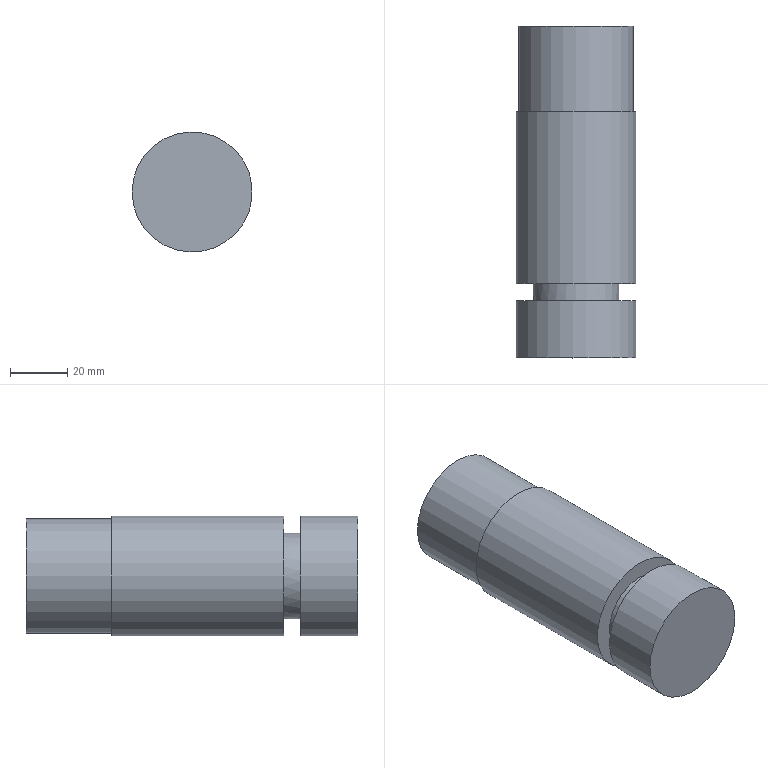Part | NX | features solid 2 | 1 solid | 9 faces | box 42 x 116 x 42 mm | volume 152776 mm3 | plane 5 | cylinder 4 | commonest cylinder face diameters 42 x2 30 x1 40 x1
STEP:
#1=CARTESIAN_POINT('',(-471.,-340.,180.));
#2=VERTEX_POINT('',#1);
#3=CARTESIAN_POINT('',(-450.,-340.,180.));
#4=DIRECTION('',(0.,1.,0.));
#5=DIRECTION('',(-1.,0.,0.));
#6=AXIS2_PLACEMENT_3D('',#3,#4,#5);
#7=CIRCLE('',#6,21.);
#8=EDGE_CURVE('',#2,#2,#7,.T.);
#9=ORIENTED_EDGE('',*,*,#8,.T.);
#10=EDGE_LOOP('',(#9));
#11=FACE_BOUND('',#10,.T.);
#12=CARTESIAN_POINT('',(-470.,-340.,180.));
#13=VERTEX_POINT('',#12);
#14=CARTESIAN_POINT('',(-450.,-340.,180.));
#15=DIRECTION('',(0.,1.,0.));
#16=DIRECTION('',(-1.,0.,0.));
#17=AXIS2_PLACEMENT_3D('',#14,#15,#16);
#18=CIRCLE('',#17,20.);
#19=EDGE_CURVE('',#13,#13,#18,.T.);
#20=ORIENTED_EDGE('',*,*,#19,.F.);
#21=EDGE_LOOP('',(#20));
#22=FACE_BOUND('',#21,.T.);
#23=CARTESIAN_POINT('',(-450.,-340.,180.));
#24=DIRECTION('',(0.,1.,0.));
#25=DIRECTION('',(0.,0.,1.));
#26=AXIS2_PLACEMENT_3D('',#23,#24,#25);
#27=PLANE('',#26);
#28=ADVANCED_FACE('',(#11,#22),#27,.T.);
#29=CARTESIAN_POINT('',(-471.,-400.,180.));
#30=VERTEX_POINT('',#29);
#31=CARTESIAN_POINT('',(-450.,-400.,180.));
#32=DIRECTION('',(0.,1.,0.));
#33=DIRECTION('',(-1.,0.,0.));
#34=AXIS2_PLACEMENT_3D('',#31,#32,#33);
#35=CIRCLE('',#34,21.);
#36=EDGE_CURVE('',#30,#30,#35,.T.);
#37=ORIENTED_EDGE('',*,*,#36,.T.);
#38=EDGE_LOOP('',(#37));
#39=FACE_BOUND('',#38,.T.);
#40=ORIENTED_EDGE('',*,*,#8,.F.);
#41=EDGE_LOOP('',(#40));
#42=FACE_BOUND('',#41,.T.);
#43=CARTESIAN_POINT('',(-450.,-400.,180.));
#44=DIRECTION('',(0.,1.,0.));
#45=DIRECTION('',(0.,0.,1.));
#46=AXIS2_PLACEMENT_3D('',#43,#44,#45);
#47=CYLINDRICAL_SURFACE('',#46,21.);
#48=ADVANCED_FACE('',(#39,#42),#47,.T.);
#49=CARTESIAN_POINT('',(-465.,-400.,180.));
#50=VERTEX_POINT('',#49);
#51=CARTESIAN_POINT('',(-450.,-400.,180.));
#52=DIRECTION('',(0.,1.,0.));
#53=DIRECTION('',(-1.,0.,0.));
#54=AXIS2_PLACEMENT_3D('',#51,#52,#53);
#55=CIRCLE('',#54,15.);
#56=EDGE_CURVE('',#50,#50,#55,.T.);
#57=ORIENTED_EDGE('',*,*,#56,.T.);
#58=EDGE_LOOP('',(#57));
#59=FACE_BOUND('',#58,.T.);
#60=ORIENTED_EDGE('',*,*,#36,.F.);
#61=EDGE_LOOP('',(#60));
#62=FACE_BOUND('',#61,.T.);
#63=CARTESIAN_POINT('',(-450.,-400.,180.));
#64=DIRECTION('',(0.,1.,0.));
#65=DIRECTION('',(0.,0.,1.));
#66=AXIS2_PLACEMENT_3D('',#63,#64,#65);
#67=PLANE('',#66);
#68=ADVANCED_FACE('',(#59,#62),#67,.F.);
#69=CARTESIAN_POINT('',(-470.,-310.,180.));
#70=VERTEX_POINT('',#69);
#71=CARTESIAN_POINT('',(-450.,-310.,180.));
#72=DIRECTION('',(0.,1.,0.));
#73=DIRECTION('',(-1.,0.,0.));
#74=AXIS2_PLACEMENT_3D('',#71,#72,#73);
#75=CIRCLE('',#74,20.);
#76=EDGE_CURVE('',#70,#70,#75,.T.);
#77=ORIENTED_EDGE('',*,*,#76,.F.);
#78=EDGE_LOOP('',(#77));
#79=FACE_BOUND('',#78,.T.);
#80=ORIENTED_EDGE('',*,*,#19,.T.);
#81=EDGE_LOOP('',(#80));
#82=FACE_BOUND('',#81,.T.);
#83=CARTESIAN_POINT('',(-450.,-310.,180.));
#84=DIRECTION('',(0.,-1.,0.));
#85=DIRECTION('',(0.,0.,-1.));
#86=AXIS2_PLACEMENT_3D('',#83,#84,#85);
#87=CYLINDRICAL_SURFACE('',#86,20.);
#88=ADVANCED_FACE('',(#79,#82),#87,.T.);
#89=ORIENTED_EDGE('',*,*,#76,.T.);
#90=EDGE_LOOP('',(#89));
#91=FACE_BOUND('',#90,.T.);
#92=CARTESIAN_POINT('',(-450.,-310.,180.));
#93=DIRECTION('',(0.,1.,0.));
#94=DIRECTION('',(0.,0.,1.));
#95=AXIS2_PLACEMENT_3D('',#92,#93,#94);
#96=PLANE('',#95);
#97=ADVANCED_FACE('',(#91),#96,.T.);
#98=CARTESIAN_POINT('',(-450.,-406.,195.));
#99=VERTEX_POINT('',#98);
#100=CARTESIAN_POINT('',(-450.,-406.,180.));
#101=DIRECTION('',(0.,1.,0.));
#102=DIRECTION('',(0.,0.,1.));
#103=AXIS2_PLACEMENT_3D('',#100,#101,#102);
#104=CIRCLE('',#103,15.);
#105=EDGE_CURVE('',#99,#99,#104,.F.);
#106=ORIENTED_EDGE('',*,*,#105,.F.);
#107=EDGE_LOOP('',(#106));
#108=FACE_BOUND('',#107,.T.);
#109=ORIENTED_EDGE('',*,*,#56,.F.);
#110=EDGE_LOOP('',(#109));
#111=FACE_BOUND('',#110,.T.);
#112=CARTESIAN_POINT('',(-450.,-406.,180.));
#113=DIRECTION('',(0.,1.,0.));
#114=DIRECTION('',(0.,0.,1.));
#115=AXIS2_PLACEMENT_3D('',#112,#113,#114);
#116=CYLINDRICAL_SURFACE('',#115,15.);
#117=ADVANCED_FACE('',(#108,#111),#116,.T.);
#118=CARTESIAN_POINT('',(-471.,-426.,180.));
#119=VERTEX_POINT('',#118);
#120=CARTESIAN_POINT('',(-450.,-426.,180.));
#121=DIRECTION('',(0.,1.,0.));
#122=DIRECTION('',(-1.,0.,0.));
#123=AXIS2_PLACEMENT_3D('',#120,#121,#122);
#124=CIRCLE('',#123,21.);
#125=EDGE_CURVE('',#119,#119,#124,.T.);
#126=ORIENTED_EDGE('',*,*,#125,.T.);
#127=EDGE_LOOP('',(#126));
#128=FACE_BOUND('',#127,.T.);
#129=CARTESIAN_POINT('',(-471.,-406.,180.));
#130=VERTEX_POINT('',#129);
#131=CARTESIAN_POINT('',(-450.,-406.,180.));
#132=DIRECTION('',(0.,1.,0.));
#133=DIRECTION('',(-1.,0.,0.));
#134=AXIS2_PLACEMENT_3D('',#131,#132,#133);
#135=CIRCLE('',#134,21.);
#136=EDGE_CURVE('',#130,#130,#135,.T.);
#137=ORIENTED_EDGE('',*,*,#136,.F.);
#138=EDGE_LOOP('',(#137));
#139=FACE_BOUND('',#138,.T.);
#140=CARTESIAN_POINT('',(-450.,-426.,180.));
#141=DIRECTION('',(0.,1.,0.));
#142=DIRECTION('',(0.,0.,1.));
#143=AXIS2_PLACEMENT_3D('',#140,#141,#142);
#144=CYLINDRICAL_SURFACE('',#143,21.);
#145=ADVANCED_FACE('',(#128,#139),#144,.T.);
#146=ORIENTED_EDGE('',*,*,#125,.F.);
#147=EDGE_LOOP('',(#146));
#148=FACE_BOUND('',#147,.T.);
#149=CARTESIAN_POINT('',(-450.,-426.,180.));
#150=DIRECTION('',(0.,1.,0.));
#151=DIRECTION('',(0.,0.,1.));
#152=AXIS2_PLACEMENT_3D('',#149,#150,#151);
#153=PLANE('',#152);
#154=ADVANCED_FACE('',(#148),#153,.F.);
#155=ORIENTED_EDGE('',*,*,#105,.T.);
#156=EDGE_LOOP('',(#155));
#157=FACE_BOUND('',#156,.T.);
#158=ORIENTED_EDGE('',*,*,#136,.T.);
#159=EDGE_LOOP('',(#158));
#160=FACE_BOUND('',#159,.T.);
#161=CARTESIAN_POINT('',(-450.,-406.,180.));
#162=DIRECTION('',(0.,1.,0.));
#163=DIRECTION('',(0.,0.,1.));
#164=AXIS2_PLACEMENT_3D('',#161,#162,#163);
#165=PLANE('',#164);
#166=ADVANCED_FACE('',(#157,#160),#165,.T.);
#167=CLOSED_SHELL('',(#28,#48,#68,#88,#97,#117,#145,#154,#166));
#168=MANIFOLD_SOLID_BREP('',#167);
#169=(LENGTH_UNIT()NAMED_UNIT(*)SI_UNIT(.MILLI.,.METRE.));
#170=UNCERTAINTY_MEASURE_WITH_UNIT(LENGTH_MEASURE(0.00001),#169,'','');
#171=(NAMED_UNIT(*)PLANE_ANGLE_UNIT()SI_UNIT($,.RADIAN.));
#172=(NAMED_UNIT(*)SI_UNIT($,.STERADIAN.)SOLID_ANGLE_UNIT());
#173=(GEOMETRIC_REPRESENTATION_CONTEXT(3)GLOBAL_UNCERTAINTY_ASSIGNED_CONTEXT((#170))GLOBAL_UNIT_ASSIGNED_CONTEXT((#169,#171,#172))REPRESENTATION_CONTEXT('',''));
#174=ADVANCED_BREP_SHAPE_REPRESENTATION('',(#168),#173);